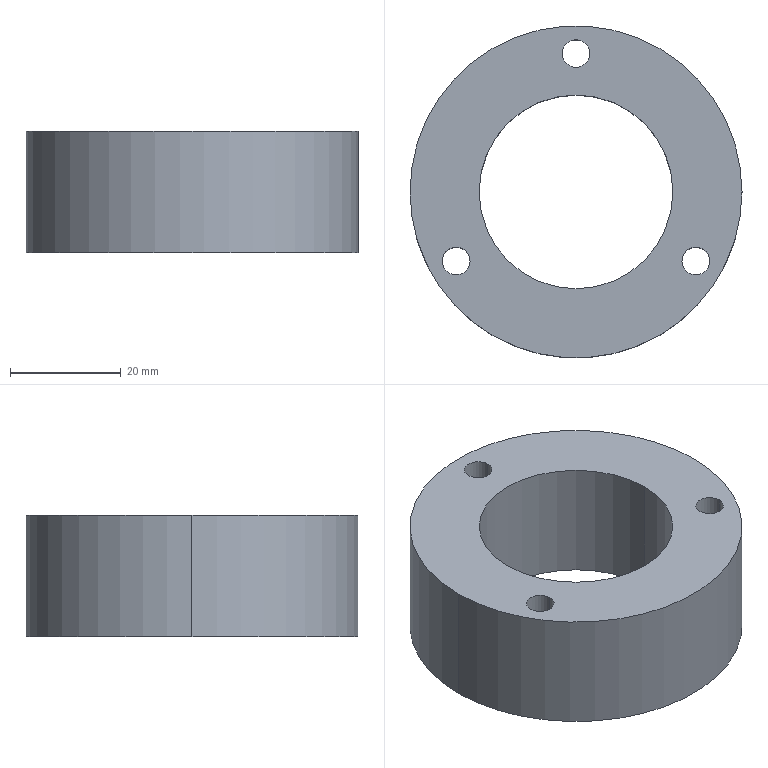Part | SolidWorks | features Extrusion 1 | 1 solid | 12 faces | box 60 x 60 x 22 mm | volume 39741 mm3 | cylinder 10 | plane 2 | commonest cylinder face diameters 5 x6 35 x2 60 x2
STEP:
#1=CARTESIAN_POINT('',(-24.151,-12.5,22.));
#2=VERTEX_POINT('',#1);
#3=CARTESIAN_POINT('',(-19.151,-12.5,22.));
#4=VERTEX_POINT('',#3);
#5=CARTESIAN_POINT('',(-21.651,-12.5,22.));
#6=DIRECTION('',(0.,0.,1.));
#7=DIRECTION('',(1.,0.,0.));
#8=AXIS2_PLACEMENT_3D('',#5,#6,#7);
#9=CIRCLE('',#8,2.5);
#10=EDGE_CURVE('',#2,#4,#9,.T.);
#11=ORIENTED_EDGE('',*,*,#10,.T.);
#12=CARTESIAN_POINT('',(-19.151,-12.5,0.));
#13=VERTEX_POINT('',#12);
#14=CARTESIAN_POINT('',(-19.151,-12.5,22.));
#15=DIRECTION('',(0.,0.,-1.));
#16=VECTOR('',#15,1000.);
#17=LINE('',#14,#16);
#18=EDGE_CURVE('',#4,#13,#17,.T.);
#19=ORIENTED_EDGE('',*,*,#18,.T.);
#20=CARTESIAN_POINT('',(-24.151,-12.5,0.));
#21=VERTEX_POINT('',#20);
#22=CARTESIAN_POINT('',(-21.651,-12.5,0.));
#23=DIRECTION('',(0.,0.,1.));
#24=DIRECTION('',(1.,0.,0.));
#25=AXIS2_PLACEMENT_3D('',#22,#23,#24);
#26=CIRCLE('',#25,2.5);
#27=EDGE_CURVE('',#21,#13,#26,.T.);
#28=ORIENTED_EDGE('',*,*,#27,.F.);
#29=CARTESIAN_POINT('',(-24.151,-12.5,22.));
#30=DIRECTION('',(0.,0.,-1.));
#31=VECTOR('',#30,1000.);
#32=LINE('',#29,#31);
#33=EDGE_CURVE('',#2,#21,#32,.T.);
#34=ORIENTED_EDGE('',*,*,#33,.F.);
#35=EDGE_LOOP('',(#11,#19,#28,#34));
#36=FACE_OUTER_BOUND('',#35,.T.);
#37=CARTESIAN_POINT('',(-21.651,-12.5,22.));
#38=DIRECTION('',(0.,0.,-1.));
#39=DIRECTION('',(-1.,0.,0.));
#40=AXIS2_PLACEMENT_3D('',#37,#38,#39);
#41=CYLINDRICAL_SURFACE('',#40,2.5);
#42=ADVANCED_FACE('',(#36),#41,.F.);
#43=CARTESIAN_POINT('',(19.151,-12.5,22.));
#44=VERTEX_POINT('',#43);
#45=CARTESIAN_POINT('',(24.151,-12.5,22.));
#46=VERTEX_POINT('',#45);
#47=CARTESIAN_POINT('',(21.651,-12.5,22.));
#48=DIRECTION('',(0.,0.,1.));
#49=DIRECTION('',(1.,0.,0.));
#50=AXIS2_PLACEMENT_3D('',#47,#48,#49);
#51=CIRCLE('',#50,2.5);
#52=EDGE_CURVE('',#44,#46,#51,.T.);
#53=ORIENTED_EDGE('',*,*,#52,.T.);
#54=CARTESIAN_POINT('',(24.151,-12.5,0.));
#55=VERTEX_POINT('',#54);
#56=CARTESIAN_POINT('',(24.151,-12.5,22.));
#57=DIRECTION('',(0.,0.,-1.));
#58=VECTOR('',#57,1000.);
#59=LINE('',#56,#58);
#60=EDGE_CURVE('',#46,#55,#59,.T.);
#61=ORIENTED_EDGE('',*,*,#60,.T.);
#62=CARTESIAN_POINT('',(19.151,-12.5,0.));
#63=VERTEX_POINT('',#62);
#64=CARTESIAN_POINT('',(21.651,-12.5,0.));
#65=DIRECTION('',(0.,0.,1.));
#66=DIRECTION('',(1.,0.,0.));
#67=AXIS2_PLACEMENT_3D('',#64,#65,#66);
#68=CIRCLE('',#67,2.5);
#69=EDGE_CURVE('',#63,#55,#68,.T.);
#70=ORIENTED_EDGE('',*,*,#69,.F.);
#71=CARTESIAN_POINT('',(19.151,-12.5,22.));
#72=DIRECTION('',(0.,0.,-1.));
#73=VECTOR('',#72,1000.);
#74=LINE('',#71,#73);
#75=EDGE_CURVE('',#44,#63,#74,.T.);
#76=ORIENTED_EDGE('',*,*,#75,.F.);
#77=EDGE_LOOP('',(#53,#61,#70,#76));
#78=FACE_OUTER_BOUND('',#77,.T.);
#79=CARTESIAN_POINT('',(21.651,-12.5,22.));
#80=DIRECTION('',(0.,0.,-1.));
#81=DIRECTION('',(-1.,0.,0.));
#82=AXIS2_PLACEMENT_3D('',#79,#80,#81);
#83=CYLINDRICAL_SURFACE('',#82,2.5);
#84=ADVANCED_FACE('',(#78),#83,.F.);
#85=CARTESIAN_POINT('',(-2.5,25.,22.));
#86=VERTEX_POINT('',#85);
#87=CARTESIAN_POINT('',(2.5,25.,22.));
#88=VERTEX_POINT('',#87);
#89=CARTESIAN_POINT('',(0.,25.,22.));
#90=DIRECTION('',(0.,0.,1.));
#91=DIRECTION('',(1.,0.,0.));
#92=AXIS2_PLACEMENT_3D('',#89,#90,#91);
#93=CIRCLE('',#92,2.5);
#94=EDGE_CURVE('',#86,#88,#93,.T.);
#95=ORIENTED_EDGE('',*,*,#94,.T.);
#96=CARTESIAN_POINT('',(2.5,25.,0.));
#97=VERTEX_POINT('',#96);
#98=CARTESIAN_POINT('',(2.5,25.,22.));
#99=DIRECTION('',(0.,0.,-1.));
#100=VECTOR('',#99,1000.);
#101=LINE('',#98,#100);
#102=EDGE_CURVE('',#88,#97,#101,.T.);
#103=ORIENTED_EDGE('',*,*,#102,.T.);
#104=CARTESIAN_POINT('',(-2.5,25.,0.));
#105=VERTEX_POINT('',#104);
#106=CARTESIAN_POINT('',(0.,25.,0.));
#107=DIRECTION('',(0.,0.,1.));
#108=DIRECTION('',(1.,0.,0.));
#109=AXIS2_PLACEMENT_3D('',#106,#107,#108);
#110=CIRCLE('',#109,2.5);
#111=EDGE_CURVE('',#105,#97,#110,.T.);
#112=ORIENTED_EDGE('',*,*,#111,.F.);
#113=CARTESIAN_POINT('',(-2.5,25.,22.));
#114=DIRECTION('',(0.,0.,-1.));
#115=VECTOR('',#114,1000.);
#116=LINE('',#113,#115);
#117=EDGE_CURVE('',#86,#105,#116,.T.);
#118=ORIENTED_EDGE('',*,*,#117,.F.);
#119=EDGE_LOOP('',(#95,#103,#112,#118));
#120=FACE_OUTER_BOUND('',#119,.T.);
#121=CARTESIAN_POINT('',(0.,25.,22.));
#122=DIRECTION('',(0.,0.,-1.));
#123=DIRECTION('',(-1.,0.,0.));
#124=AXIS2_PLACEMENT_3D('',#121,#122,#123);
#125=CYLINDRICAL_SURFACE('',#124,2.5);
#126=ADVANCED_FACE('',(#120),#125,.F.);
#127=CARTESIAN_POINT('',(-17.5,0.,22.));
#128=VERTEX_POINT('',#127);
#129=CARTESIAN_POINT('',(17.5,0.,22.));
#130=VERTEX_POINT('',#129);
#131=CARTESIAN_POINT('',(0.,0.,22.));
#132=DIRECTION('',(0.,0.,1.));
#133=DIRECTION('',(1.,0.,0.));
#134=AXIS2_PLACEMENT_3D('',#131,#132,#133);
#135=CIRCLE('',#134,17.5);
#136=EDGE_CURVE('',#128,#130,#135,.T.);
#137=ORIENTED_EDGE('',*,*,#136,.T.);
#138=CARTESIAN_POINT('',(17.5,0.,0.));
#139=VERTEX_POINT('',#138);
#140=CARTESIAN_POINT('',(17.5,0.,22.));
#141=DIRECTION('',(0.,0.,-1.));
#142=VECTOR('',#141,1000.);
#143=LINE('',#140,#142);
#144=EDGE_CURVE('',#130,#139,#143,.T.);
#145=ORIENTED_EDGE('',*,*,#144,.T.);
#146=CARTESIAN_POINT('',(-17.5,0.,0.));
#147=VERTEX_POINT('',#146);
#148=CARTESIAN_POINT('',(0.,0.,0.));
#149=DIRECTION('',(0.,0.,1.));
#150=DIRECTION('',(1.,0.,0.));
#151=AXIS2_PLACEMENT_3D('',#148,#149,#150);
#152=CIRCLE('',#151,17.5);
#153=EDGE_CURVE('',#147,#139,#152,.T.);
#154=ORIENTED_EDGE('',*,*,#153,.F.);
#155=CARTESIAN_POINT('',(-17.5,0.,22.));
#156=DIRECTION('',(0.,0.,-1.));
#157=VECTOR('',#156,1000.);
#158=LINE('',#155,#157);
#159=EDGE_CURVE('',#128,#147,#158,.T.);
#160=ORIENTED_EDGE('',*,*,#159,.F.);
#161=EDGE_LOOP('',(#137,#145,#154,#160));
#162=FACE_OUTER_BOUND('',#161,.T.);
#163=CARTESIAN_POINT('',(0.,0.,22.));
#164=DIRECTION('',(0.,0.,-1.));
#165=DIRECTION('',(-1.,0.,0.));
#166=AXIS2_PLACEMENT_3D('',#163,#164,#165);
#167=CYLINDRICAL_SURFACE('',#166,17.5);
#168=ADVANCED_FACE('',(#162),#167,.F.);
#169=CARTESIAN_POINT('',(30.,0.,22.));
#170=VERTEX_POINT('',#169);
#171=CARTESIAN_POINT('',(-30.,0.,22.));
#172=VERTEX_POINT('',#171);
#173=CARTESIAN_POINT('',(0.,0.,22.));
#174=DIRECTION('',(0.,0.,1.));
#175=DIRECTION('',(1.,0.,0.));
#176=AXIS2_PLACEMENT_3D('',#173,#174,#175);
#177=CIRCLE('',#176,30.);
#178=EDGE_CURVE('',#170,#172,#177,.T.);
#179=ORIENTED_EDGE('',*,*,#178,.F.);
#180=CARTESIAN_POINT('',(30.,0.,0.));
#181=VERTEX_POINT('',#180);
#182=CARTESIAN_POINT('',(30.,0.,22.));
#183=DIRECTION('',(0.,0.,-1.));
#184=VECTOR('',#183,1000.);
#185=LINE('',#182,#184);
#186=EDGE_CURVE('',#170,#181,#185,.T.);
#187=ORIENTED_EDGE('',*,*,#186,.T.);
#188=CARTESIAN_POINT('',(-30.,0.,0.));
#189=VERTEX_POINT('',#188);
#190=CARTESIAN_POINT('',(0.,0.,0.));
#191=DIRECTION('',(0.,0.,1.));
#192=DIRECTION('',(1.,0.,0.));
#193=AXIS2_PLACEMENT_3D('',#190,#191,#192);
#194=CIRCLE('',#193,30.);
#195=EDGE_CURVE('',#181,#189,#194,.T.);
#196=ORIENTED_EDGE('',*,*,#195,.T.);
#197=CARTESIAN_POINT('',(-30.,0.,22.));
#198=DIRECTION('',(0.,0.,-1.));
#199=VECTOR('',#198,1000.);
#200=LINE('',#197,#199);
#201=EDGE_CURVE('',#172,#189,#200,.T.);
#202=ORIENTED_EDGE('',*,*,#201,.F.);
#203=EDGE_LOOP('',(#179,#187,#196,#202));
#204=FACE_OUTER_BOUND('',#203,.T.);
#205=CARTESIAN_POINT('',(0.,0.,22.));
#206=DIRECTION('',(0.,0.,-1.));
#207=DIRECTION('',(-1.,0.,0.));
#208=AXIS2_PLACEMENT_3D('',#205,#206,#207);
#209=CYLINDRICAL_SURFACE('',#208,30.);
#210=ADVANCED_FACE('',(#204),#209,.T.);
#211=ORIENTED_EDGE('',*,*,#52,.F.);
#212=CARTESIAN_POINT('',(21.651,-12.5,22.));
#213=DIRECTION('',(0.,0.,1.));
#214=DIRECTION('',(1.,0.,0.));
#215=AXIS2_PLACEMENT_3D('',#212,#213,#214);
#216=CIRCLE('',#215,2.5);
#217=EDGE_CURVE('',#46,#44,#216,.T.);
#218=ORIENTED_EDGE('',*,*,#217,.F.);
#219=EDGE_LOOP('',(#211,#218));
#220=FACE_BOUND('',#219,.T.);
#221=ORIENTED_EDGE('',*,*,#136,.F.);
#222=CARTESIAN_POINT('',(0.,0.,22.));
#223=DIRECTION('',(0.,0.,1.));
#224=DIRECTION('',(1.,0.,0.));
#225=AXIS2_PLACEMENT_3D('',#222,#223,#224);
#226=CIRCLE('',#225,17.5);
#227=EDGE_CURVE('',#130,#128,#226,.T.);
#228=ORIENTED_EDGE('',*,*,#227,.F.);
#229=EDGE_LOOP('',(#221,#228));
#230=FACE_BOUND('',#229,.T.);
#231=CARTESIAN_POINT('',(0.,0.,22.));
#232=DIRECTION('',(0.,0.,1.));
#233=DIRECTION('',(1.,0.,0.));
#234=AXIS2_PLACEMENT_3D('',#231,#232,#233);
#235=CIRCLE('',#234,30.);
#236=EDGE_CURVE('',#172,#170,#235,.T.);
#237=ORIENTED_EDGE('',*,*,#236,.T.);
#238=ORIENTED_EDGE('',*,*,#178,.T.);
#239=EDGE_LOOP('',(#237,#238));
#240=FACE_OUTER_BOUND('',#239,.T.);
#241=ORIENTED_EDGE('',*,*,#94,.F.);
#242=CARTESIAN_POINT('',(0.,25.,22.));
#243=DIRECTION('',(0.,0.,1.));
#244=DIRECTION('',(1.,0.,0.));
#245=AXIS2_PLACEMENT_3D('',#242,#243,#244);
#246=CIRCLE('',#245,2.5);
#247=EDGE_CURVE('',#88,#86,#246,.T.);
#248=ORIENTED_EDGE('',*,*,#247,.F.);
#249=EDGE_LOOP('',(#241,#248));
#250=FACE_BOUND('',#249,.T.);
#251=ORIENTED_EDGE('',*,*,#10,.F.);
#252=CARTESIAN_POINT('',(-21.651,-12.5,22.));
#253=DIRECTION('',(0.,0.,1.));
#254=DIRECTION('',(1.,0.,0.));
#255=AXIS2_PLACEMENT_3D('',#252,#253,#254);
#256=CIRCLE('',#255,2.5);
#257=EDGE_CURVE('',#4,#2,#256,.T.);
#258=ORIENTED_EDGE('',*,*,#257,.F.);
#259=EDGE_LOOP('',(#251,#258));
#260=FACE_BOUND('',#259,.T.);
#261=CARTESIAN_POINT('',(0.,0.,22.));
#262=DIRECTION('',(0.,0.,1.));
#263=DIRECTION('',(1.,0.,0.));
#264=AXIS2_PLACEMENT_3D('',#261,#262,#263);
#265=PLANE('',#264);
#266=ADVANCED_FACE('',(#220,#230,#240,#250,#260),#265,.T.);
#267=CARTESIAN_POINT('',(0.,0.,0.));
#268=DIRECTION('',(0.,0.,1.));
#269=DIRECTION('',(1.,0.,0.));
#270=AXIS2_PLACEMENT_3D('',#267,#268,#269);
#271=CIRCLE('',#270,30.);
#272=EDGE_CURVE('',#189,#181,#271,.T.);
#273=ORIENTED_EDGE('',*,*,#272,.F.);
#274=ORIENTED_EDGE('',*,*,#195,.F.);
#275=EDGE_LOOP('',(#273,#274));
#276=FACE_OUTER_BOUND('',#275,.T.);
#277=ORIENTED_EDGE('',*,*,#153,.T.);
#278=CARTESIAN_POINT('',(0.,0.,0.));
#279=DIRECTION('',(0.,0.,1.));
#280=DIRECTION('',(1.,0.,0.));
#281=AXIS2_PLACEMENT_3D('',#278,#279,#280);
#282=CIRCLE('',#281,17.5);
#283=EDGE_CURVE('',#139,#147,#282,.T.);
#284=ORIENTED_EDGE('',*,*,#283,.T.);
#285=EDGE_LOOP('',(#277,#284));
#286=FACE_BOUND('',#285,.T.);
#287=ORIENTED_EDGE('',*,*,#111,.T.);
#288=CARTESIAN_POINT('',(0.,25.,0.));
#289=DIRECTION('',(0.,0.,1.));
#290=DIRECTION('',(1.,0.,0.));
#291=AXIS2_PLACEMENT_3D('',#288,#289,#290);
#292=CIRCLE('',#291,2.5);
#293=EDGE_CURVE('',#97,#105,#292,.T.);
#294=ORIENTED_EDGE('',*,*,#293,.T.);
#295=EDGE_LOOP('',(#287,#294));
#296=FACE_BOUND('',#295,.T.);
#297=ORIENTED_EDGE('',*,*,#69,.T.);
#298=CARTESIAN_POINT('',(21.651,-12.5,0.));
#299=DIRECTION('',(0.,0.,1.));
#300=DIRECTION('',(1.,0.,0.));
#301=AXIS2_PLACEMENT_3D('',#298,#299,#300);
#302=CIRCLE('',#301,2.5);
#303=EDGE_CURVE('',#55,#63,#302,.T.);
#304=ORIENTED_EDGE('',*,*,#303,.T.);
#305=EDGE_LOOP('',(#297,#304));
#306=FACE_BOUND('',#305,.T.);
#307=ORIENTED_EDGE('',*,*,#27,.T.);
#308=CARTESIAN_POINT('',(-21.651,-12.5,0.));
#309=DIRECTION('',(0.,0.,1.));
#310=DIRECTION('',(1.,0.,0.));
#311=AXIS2_PLACEMENT_3D('',#308,#309,#310);
#312=CIRCLE('',#311,2.5);
#313=EDGE_CURVE('',#13,#21,#312,.T.);
#314=ORIENTED_EDGE('',*,*,#313,.T.);
#315=EDGE_LOOP('',(#307,#314));
#316=FACE_BOUND('',#315,.T.);
#317=CARTESIAN_POINT('',(0.,0.,0.));
#318=DIRECTION('',(0.,0.,1.));
#319=DIRECTION('',(1.,0.,0.));
#320=AXIS2_PLACEMENT_3D('',#317,#318,#319);
#321=PLANE('',#320);
#322=ADVANCED_FACE('',(#276,#286,#296,#306,#316),#321,.F.);
#323=ORIENTED_EDGE('',*,*,#186,.F.);
#324=ORIENTED_EDGE('',*,*,#236,.F.);
#325=ORIENTED_EDGE('',*,*,#201,.T.);
#326=ORIENTED_EDGE('',*,*,#272,.T.);
#327=EDGE_LOOP('',(#323,#324,#325,#326));
#328=FACE_OUTER_BOUND('',#327,.T.);
#329=CARTESIAN_POINT('',(0.,0.,22.));
#330=DIRECTION('',(0.,0.,-1.));
#331=DIRECTION('',(-1.,0.,0.));
#332=AXIS2_PLACEMENT_3D('',#329,#330,#331);
#333=CYLINDRICAL_SURFACE('',#332,30.);
#334=ADVANCED_FACE('',(#328),#333,.T.);
#335=ORIENTED_EDGE('',*,*,#144,.F.);
#336=ORIENTED_EDGE('',*,*,#227,.T.);
#337=ORIENTED_EDGE('',*,*,#159,.T.);
#338=ORIENTED_EDGE('',*,*,#283,.F.);
#339=EDGE_LOOP('',(#335,#336,#337,#338));
#340=FACE_OUTER_BOUND('',#339,.T.);
#341=CARTESIAN_POINT('',(0.,0.,22.));
#342=DIRECTION('',(0.,0.,-1.));
#343=DIRECTION('',(-1.,0.,0.));
#344=AXIS2_PLACEMENT_3D('',#341,#342,#343);
#345=CYLINDRICAL_SURFACE('',#344,17.5);
#346=ADVANCED_FACE('',(#340),#345,.F.);
#347=ORIENTED_EDGE('',*,*,#102,.F.);
#348=ORIENTED_EDGE('',*,*,#247,.T.);
#349=ORIENTED_EDGE('',*,*,#117,.T.);
#350=ORIENTED_EDGE('',*,*,#293,.F.);
#351=EDGE_LOOP('',(#347,#348,#349,#350));
#352=FACE_OUTER_BOUND('',#351,.T.);
#353=CARTESIAN_POINT('',(0.,25.,22.));
#354=DIRECTION('',(0.,0.,-1.));
#355=DIRECTION('',(-1.,0.,0.));
#356=AXIS2_PLACEMENT_3D('',#353,#354,#355);
#357=CYLINDRICAL_SURFACE('',#356,2.5);
#358=ADVANCED_FACE('',(#352),#357,.F.);
#359=ORIENTED_EDGE('',*,*,#60,.F.);
#360=ORIENTED_EDGE('',*,*,#217,.T.);
#361=ORIENTED_EDGE('',*,*,#75,.T.);
#362=ORIENTED_EDGE('',*,*,#303,.F.);
#363=EDGE_LOOP('',(#359,#360,#361,#362));
#364=FACE_OUTER_BOUND('',#363,.T.);
#365=CARTESIAN_POINT('',(21.651,-12.5,22.));
#366=DIRECTION('',(0.,0.,-1.));
#367=DIRECTION('',(-1.,0.,0.));
#368=AXIS2_PLACEMENT_3D('',#365,#366,#367);
#369=CYLINDRICAL_SURFACE('',#368,2.5);
#370=ADVANCED_FACE('',(#364),#369,.F.);
#371=ORIENTED_EDGE('',*,*,#18,.F.);
#372=ORIENTED_EDGE('',*,*,#257,.T.);
#373=ORIENTED_EDGE('',*,*,#33,.T.);
#374=ORIENTED_EDGE('',*,*,#313,.F.);
#375=EDGE_LOOP('',(#371,#372,#373,#374));
#376=FACE_OUTER_BOUND('',#375,.T.);
#377=CARTESIAN_POINT('',(-21.651,-12.5,22.));
#378=DIRECTION('',(0.,0.,-1.));
#379=DIRECTION('',(-1.,0.,0.));
#380=AXIS2_PLACEMENT_3D('',#377,#378,#379);
#381=CYLINDRICAL_SURFACE('',#380,2.5);
#382=ADVANCED_FACE('',(#376),#381,.F.);
#383=CLOSED_SHELL('',(#42,#84,#126,#168,#210,#266,#322,#334,#346,#358,#370,#382));
#384=MANIFOLD_SOLID_BREP('',#383);
#385=CARTESIAN_POINT('',(0.,0.,0.));
#386=DIRECTION('',(0.,0.,1.));
#387=DIRECTION('',(1.,0.,0.));
#388=AXIS2_PLACEMENT_3D('',#385,#386,#387);
#389=(LENGTH_UNIT()NAMED_UNIT(*)SI_UNIT(.MILLI.,.METRE.));
#390=UNCERTAINTY_MEASURE_WITH_UNIT(LENGTH_MEASURE(0.00001),#389,'','');
#391=(NAMED_UNIT(*)PLANE_ANGLE_UNIT()SI_UNIT($,.RADIAN.));
#392=(NAMED_UNIT(*)SI_UNIT($,.STERADIAN.)SOLID_ANGLE_UNIT());
#393=(GEOMETRIC_REPRESENTATION_CONTEXT(3)GLOBAL_UNCERTAINTY_ASSIGNED_CONTEXT((#390))GLOBAL_UNIT_ASSIGNED_CONTEXT((#389,#391,#392))REPRESENTATION_CONTEXT('',''));
#394=ADVANCED_BREP_SHAPE_REPRESENTATION('',(#384,#388),#393);